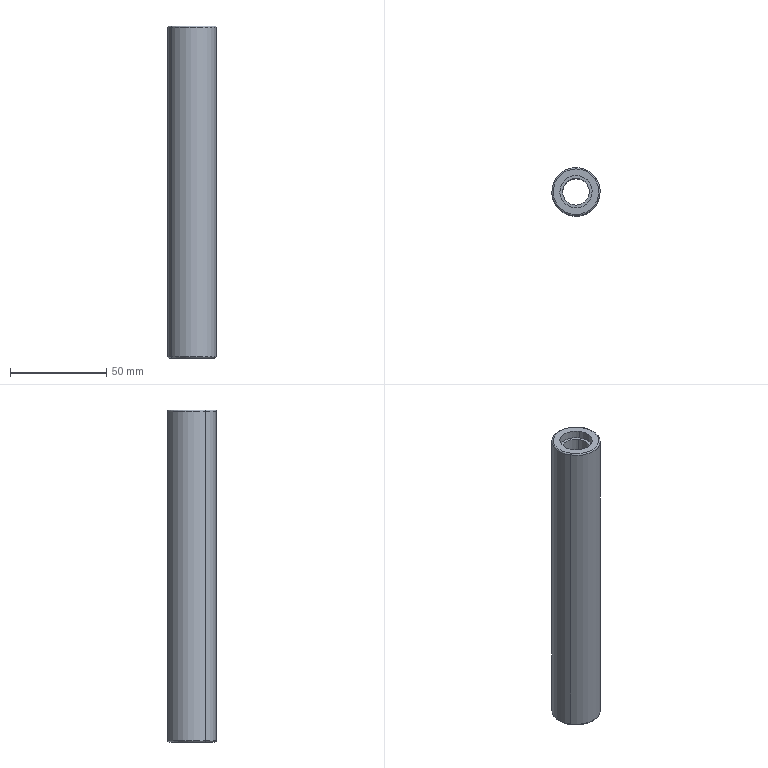Part | SolidWorks | features SplitBody 1 | 1 solid | 16 faces | box 25.2 x 25.2 x 172.9 mm | volume 59034 mm3 | cylinder 8 | torus 4 | plane 4 | commonest cylinder face diameters 16.8 x4 14 x2 25.2 x2
STEP:
#1=CARTESIAN_POINT('',(443.484,236.395,-446.666));
#2=VERTEX_POINT('',#1);
#3=CARTESIAN_POINT('',(463.467,249.323,-446.666));
#4=VERTEX_POINT('',#3);
#5=CARTESIAN_POINT('',(453.475,242.859,-446.666));
#6=DIRECTION('',(0.,0.,-1.));
#7=DIRECTION('',(0.8396,0.5432,0.));
#8=AXIS2_PLACEMENT_3D('',#5,#6,#7);
#9=CIRCLE('',#8,11.9);
#10=EDGE_CURVE('',#2,#4,#9,.T.);
#11=ORIENTED_EDGE('',*,*,#10,.F.);
#12=CARTESIAN_POINT('',(442.896,236.015,-445.966));
#13=VERTEX_POINT('',#12);
#14=CARTESIAN_POINT('',(443.484,236.395,-445.966));
#15=DIRECTION('',(-0.5432,0.8396,0.));
#16=DIRECTION('',(-0.8396,-0.5432,0.));
#17=AXIS2_PLACEMENT_3D('',#14,#15,#16);
#18=CIRCLE('',#17,0.7);
#19=EDGE_CURVE('',#2,#13,#18,.T.);
#20=ORIENTED_EDGE('',*,*,#19,.T.);
#21=CARTESIAN_POINT('',(464.055,249.703,-445.966));
#22=VERTEX_POINT('',#21);
#23=CARTESIAN_POINT('',(453.475,242.859,-445.966));
#24=DIRECTION('',(0.,0.,1.));
#25=DIRECTION('',(0.8396,0.5432,0.));
#26=AXIS2_PLACEMENT_3D('',#23,#24,#25);
#27=CIRCLE('',#26,12.6);
#28=EDGE_CURVE('',#22,#13,#27,.T.);
#29=ORIENTED_EDGE('',*,*,#28,.F.);
#30=CARTESIAN_POINT('',(463.467,249.323,-445.966));
#31=DIRECTION('',(0.5432,-0.8396,0.));
#32=DIRECTION('',(0.8396,0.5432,0.));
#33=AXIS2_PLACEMENT_3D('',#30,#31,#32);
#34=CIRCLE('',#33,0.7);
#35=EDGE_CURVE('',#4,#22,#34,.T.);
#36=ORIENTED_EDGE('',*,*,#35,.F.);
#37=EDGE_LOOP('',(#11,#20,#29,#36));
#38=FACE_OUTER_BOUND('',#37,.T.);
#39=CARTESIAN_POINT('',(453.475,242.859,-445.966));
#40=DIRECTION('',(0.,0.,1.));
#41=DIRECTION('',(0.8396,0.5432,0.));
#42=AXIS2_PLACEMENT_3D('',#39,#40,#41);
#43=TOROIDAL_SURFACE('',#42,11.9,0.7);
#44=ADVANCED_FACE('',(#38),#43,.T.);
#45=CARTESIAN_POINT('',(442.896,236.015,-274.466));
#46=VERTEX_POINT('',#45);
#47=CARTESIAN_POINT('',(464.055,249.703,-274.466));
#48=VERTEX_POINT('',#47);
#49=CARTESIAN_POINT('',(453.475,242.859,-274.466));
#50=DIRECTION('',(0.,0.,-1.));
#51=DIRECTION('',(0.8396,0.5432,0.));
#52=AXIS2_PLACEMENT_3D('',#49,#50,#51);
#53=CIRCLE('',#52,12.6);
#54=EDGE_CURVE('',#46,#48,#53,.T.);
#55=ORIENTED_EDGE('',*,*,#54,.F.);
#56=CARTESIAN_POINT('',(443.484,236.395,-273.766));
#57=VERTEX_POINT('',#56);
#58=CARTESIAN_POINT('',(443.484,236.395,-274.466));
#59=DIRECTION('',(-0.5432,0.8396,0.));
#60=DIRECTION('',(-0.8396,-0.5432,0.));
#61=AXIS2_PLACEMENT_3D('',#58,#59,#60);
#62=CIRCLE('',#61,0.7);
#63=EDGE_CURVE('',#46,#57,#62,.T.);
#64=ORIENTED_EDGE('',*,*,#63,.T.);
#65=CARTESIAN_POINT('',(463.467,249.323,-273.766));
#66=VERTEX_POINT('',#65);
#67=CARTESIAN_POINT('',(453.475,242.859,-273.766));
#68=DIRECTION('',(0.,0.,1.));
#69=DIRECTION('',(0.8396,0.5432,0.));
#70=AXIS2_PLACEMENT_3D('',#67,#68,#69);
#71=CIRCLE('',#70,11.9);
#72=EDGE_CURVE('',#66,#57,#71,.T.);
#73=ORIENTED_EDGE('',*,*,#72,.F.);
#74=CARTESIAN_POINT('',(463.467,249.323,-274.466));
#75=DIRECTION('',(0.5432,-0.8396,0.));
#76=DIRECTION('',(0.8396,0.5432,0.));
#77=AXIS2_PLACEMENT_3D('',#74,#75,#76);
#78=CIRCLE('',#77,0.7);
#79=EDGE_CURVE('',#48,#66,#78,.T.);
#80=ORIENTED_EDGE('',*,*,#79,.F.);
#81=EDGE_LOOP('',(#55,#64,#73,#80));
#82=FACE_OUTER_BOUND('',#81,.T.);
#83=CARTESIAN_POINT('',(453.475,242.859,-274.466));
#84=DIRECTION('',(0.,0.,1.));
#85=DIRECTION('',(0.8396,0.5432,0.));
#86=AXIS2_PLACEMENT_3D('',#83,#84,#85);
#87=TOROIDAL_SURFACE('',#86,11.9,0.7);
#88=ADVANCED_FACE('',(#82),#87,.T.);
#89=CARTESIAN_POINT('',(447.598,239.057,-277.966));
#90=VERTEX_POINT('',#89);
#91=CARTESIAN_POINT('',(459.353,246.661,-277.966));
#92=VERTEX_POINT('',#91);
#93=CARTESIAN_POINT('',(453.475,242.859,-277.966));
#94=DIRECTION('',(0.,0.,1.));
#95=DIRECTION('',(0.8396,0.5432,0.));
#96=AXIS2_PLACEMENT_3D('',#93,#94,#95);
#97=CIRCLE('',#96,7.);
#98=EDGE_CURVE('',#90,#92,#97,.T.);
#99=ORIENTED_EDGE('',*,*,#98,.T.);
#100=CARTESIAN_POINT('',(459.353,246.661,-442.466));
#101=VERTEX_POINT('',#100);
#102=CARTESIAN_POINT('',(459.353,246.661,-273.766));
#103=DIRECTION('',(0.,0.,-1.));
#104=VECTOR('',#103,1000.);
#105=LINE('',#102,#104);
#106=EDGE_CURVE('',#92,#101,#105,.T.);
#107=ORIENTED_EDGE('',*,*,#106,.T.);
#108=CARTESIAN_POINT('',(447.598,239.057,-442.466));
#109=VERTEX_POINT('',#108);
#110=CARTESIAN_POINT('',(453.475,242.859,-442.466));
#111=DIRECTION('',(0.,0.,-1.));
#112=DIRECTION('',(-0.8396,-0.5432,0.));
#113=AXIS2_PLACEMENT_3D('',#110,#111,#112);
#114=CIRCLE('',#113,7.);
#115=EDGE_CURVE('',#101,#109,#114,.T.);
#116=ORIENTED_EDGE('',*,*,#115,.T.);
#117=CARTESIAN_POINT('',(447.598,239.057,-273.766));
#118=DIRECTION('',(0.,0.,-1.));
#119=VECTOR('',#118,1000.);
#120=LINE('',#117,#119);
#121=EDGE_CURVE('',#90,#109,#120,.T.);
#122=ORIENTED_EDGE('',*,*,#121,.F.);
#123=EDGE_LOOP('',(#99,#107,#116,#122));
#124=FACE_OUTER_BOUND('',#123,.T.);
#125=CARTESIAN_POINT('',(453.475,242.859,-273.766));
#126=DIRECTION('',(0.,0.,-1.));
#127=DIRECTION('',(-0.8396,-0.5432,0.));
#128=AXIS2_PLACEMENT_3D('',#125,#126,#127);
#129=CYLINDRICAL_SURFACE('',#128,7.);
#130=ADVANCED_FACE('',(#124),#129,.F.);
#131=CARTESIAN_POINT('',(460.528,247.422,-442.466));
#132=VERTEX_POINT('',#131);
#133=CARTESIAN_POINT('',(446.423,238.296,-442.466));
#134=VERTEX_POINT('',#133);
#135=CARTESIAN_POINT('',(453.475,242.859,-442.466));
#136=DIRECTION('',(0.,0.,-1.));
#137=DIRECTION('',(-0.8396,-0.5432,0.));
#138=AXIS2_PLACEMENT_3D('',#135,#136,#137);
#139=CIRCLE('',#138,8.4);
#140=EDGE_CURVE('',#132,#134,#139,.T.);
#141=ORIENTED_EDGE('',*,*,#140,.F.);
#142=CARTESIAN_POINT('',(460.528,247.422,-446.666));
#143=VERTEX_POINT('',#142);
#144=CARTESIAN_POINT('',(460.528,247.422,-442.466));
#145=DIRECTION('',(0.,0.,-1.));
#146=VECTOR('',#145,1000.);
#147=LINE('',#144,#146);
#148=EDGE_CURVE('',#132,#143,#147,.T.);
#149=ORIENTED_EDGE('',*,*,#148,.T.);
#150=CARTESIAN_POINT('',(446.423,238.296,-446.666));
#151=VERTEX_POINT('',#150);
#152=CARTESIAN_POINT('',(453.475,242.859,-446.666));
#153=DIRECTION('',(0.,0.,-1.));
#154=DIRECTION('',(-0.8396,-0.5432,0.));
#155=AXIS2_PLACEMENT_3D('',#152,#153,#154);
#156=CIRCLE('',#155,8.4);
#157=EDGE_CURVE('',#143,#151,#156,.T.);
#158=ORIENTED_EDGE('',*,*,#157,.T.);
#159=CARTESIAN_POINT('',(446.423,238.296,-442.466));
#160=DIRECTION('',(0.,0.,-1.));
#161=VECTOR('',#160,1000.);
#162=LINE('',#159,#161);
#163=EDGE_CURVE('',#134,#151,#162,.T.);
#164=ORIENTED_EDGE('',*,*,#163,.F.);
#165=EDGE_LOOP('',(#141,#149,#158,#164));
#166=FACE_OUTER_BOUND('',#165,.T.);
#167=CARTESIAN_POINT('',(453.475,242.859,-442.466));
#168=DIRECTION('',(0.,0.,-1.));
#169=DIRECTION('',(-0.8396,-0.5432,0.));
#170=AXIS2_PLACEMENT_3D('',#167,#168,#169);
#171=CYLINDRICAL_SURFACE('',#170,8.4);
#172=ADVANCED_FACE('',(#166),#171,.F.);
#173=CARTESIAN_POINT('',(446.423,238.296,-277.966));
#174=VERTEX_POINT('',#173);
#175=CARTESIAN_POINT('',(460.528,247.422,-277.966));
#176=VERTEX_POINT('',#175);
#177=CARTESIAN_POINT('',(453.475,242.859,-277.966));
#178=DIRECTION('',(0.,0.,1.));
#179=DIRECTION('',(0.8396,0.5432,0.));
#180=AXIS2_PLACEMENT_3D('',#177,#178,#179);
#181=CIRCLE('',#180,8.4);
#182=EDGE_CURVE('',#174,#176,#181,.T.);
#183=ORIENTED_EDGE('',*,*,#182,.F.);
#184=CARTESIAN_POINT('',(446.423,238.296,-273.766));
#185=VERTEX_POINT('',#184);
#186=CARTESIAN_POINT('',(446.423,238.296,-277.966));
#187=DIRECTION('',(0.,0.,1.));
#188=VECTOR('',#187,1000.);
#189=LINE('',#186,#188);
#190=EDGE_CURVE('',#174,#185,#189,.T.);
#191=ORIENTED_EDGE('',*,*,#190,.T.);
#192=CARTESIAN_POINT('',(460.528,247.422,-273.766));
#193=VERTEX_POINT('',#192);
#194=CARTESIAN_POINT('',(453.475,242.859,-273.766));
#195=DIRECTION('',(0.,0.,1.));
#196=DIRECTION('',(0.8396,0.5432,0.));
#197=AXIS2_PLACEMENT_3D('',#194,#195,#196);
#198=CIRCLE('',#197,8.4);
#199=EDGE_CURVE('',#185,#193,#198,.T.);
#200=ORIENTED_EDGE('',*,*,#199,.T.);
#201=CARTESIAN_POINT('',(460.528,247.422,-277.966));
#202=DIRECTION('',(0.,0.,1.));
#203=VECTOR('',#202,1000.);
#204=LINE('',#201,#203);
#205=EDGE_CURVE('',#176,#193,#204,.T.);
#206=ORIENTED_EDGE('',*,*,#205,.F.);
#207=EDGE_LOOP('',(#183,#191,#200,#206));
#208=FACE_OUTER_BOUND('',#207,.T.);
#209=CARTESIAN_POINT('',(453.475,242.859,-277.966));
#210=DIRECTION('',(0.,0.,1.));
#211=DIRECTION('',(0.8396,0.5432,0.));
#212=AXIS2_PLACEMENT_3D('',#209,#210,#211);
#213=CYLINDRICAL_SURFACE('',#212,8.4);
#214=ADVANCED_FACE('',(#208),#213,.F.);
#215=ORIENTED_EDGE('',*,*,#54,.T.);
#216=CARTESIAN_POINT('',(464.055,249.703,-273.766));
#217=DIRECTION('',(0.,0.,-1.));
#218=VECTOR('',#217,1000.);
#219=LINE('',#216,#218);
#220=EDGE_CURVE('',#48,#22,#219,.T.);
#221=ORIENTED_EDGE('',*,*,#220,.T.);
#222=ORIENTED_EDGE('',*,*,#28,.T.);
#223=CARTESIAN_POINT('',(442.896,236.015,-273.766));
#224=DIRECTION('',(0.,0.,-1.));
#225=VECTOR('',#224,1000.);
#226=LINE('',#223,#225);
#227=EDGE_CURVE('',#46,#13,#226,.T.);
#228=ORIENTED_EDGE('',*,*,#227,.F.);
#229=EDGE_LOOP('',(#215,#221,#222,#228));
#230=FACE_OUTER_BOUND('',#229,.T.);
#231=CARTESIAN_POINT('',(453.475,242.859,-273.766));
#232=DIRECTION('',(0.,0.,-1.));
#233=DIRECTION('',(-0.8396,-0.5432,0.));
#234=AXIS2_PLACEMENT_3D('',#231,#232,#233);
#235=CYLINDRICAL_SURFACE('',#234,12.6);
#236=ADVANCED_FACE('',(#230),#235,.T.);
#237=ORIENTED_EDGE('',*,*,#220,.F.);
#238=CARTESIAN_POINT('',(453.475,242.859,-274.466));
#239=DIRECTION('',(0.,0.,-1.));
#240=DIRECTION('',(0.8396,0.5432,0.));
#241=AXIS2_PLACEMENT_3D('',#238,#239,#240);
#242=CIRCLE('',#241,12.6);
#243=EDGE_CURVE('',#48,#46,#242,.T.);
#244=ORIENTED_EDGE('',*,*,#243,.T.);
#245=ORIENTED_EDGE('',*,*,#227,.T.);
#246=CARTESIAN_POINT('',(453.475,242.859,-445.966));
#247=DIRECTION('',(0.,0.,1.));
#248=DIRECTION('',(0.8396,0.5432,0.));
#249=AXIS2_PLACEMENT_3D('',#246,#247,#248);
#250=CIRCLE('',#249,12.6);
#251=EDGE_CURVE('',#13,#22,#250,.T.);
#252=ORIENTED_EDGE('',*,*,#251,.T.);
#253=EDGE_LOOP('',(#237,#244,#245,#252));
#254=FACE_OUTER_BOUND('',#253,.T.);
#255=CARTESIAN_POINT('',(453.475,242.859,-273.766));
#256=DIRECTION('',(0.,0.,-1.));
#257=DIRECTION('',(-0.8396,-0.5432,0.));
#258=AXIS2_PLACEMENT_3D('',#255,#256,#257);
#259=CYLINDRICAL_SURFACE('',#258,12.6);
#260=ADVANCED_FACE('',(#254),#259,.T.);
#261=ORIENTED_EDGE('',*,*,#72,.T.);
#262=CARTESIAN_POINT('',(453.475,242.859,-273.766));
#263=DIRECTION('',(0.,0.,1.));
#264=DIRECTION('',(0.8396,0.5432,0.));
#265=AXIS2_PLACEMENT_3D('',#262,#263,#264);
#266=CIRCLE('',#265,11.9);
#267=EDGE_CURVE('',#57,#66,#266,.T.);
#268=ORIENTED_EDGE('',*,*,#267,.T.);
#269=EDGE_LOOP('',(#261,#268));
#270=FACE_OUTER_BOUND('',#269,.T.);
#271=CARTESIAN_POINT('',(453.475,242.859,-273.766));
#272=DIRECTION('',(0.,0.,1.));
#273=DIRECTION('',(0.8396,0.5432,0.));
#274=AXIS2_PLACEMENT_3D('',#271,#272,#273);
#275=CIRCLE('',#274,8.4);
#276=EDGE_CURVE('',#193,#185,#275,.T.);
#277=ORIENTED_EDGE('',*,*,#276,.F.);
#278=ORIENTED_EDGE('',*,*,#199,.F.);
#279=EDGE_LOOP('',(#277,#278));
#280=FACE_BOUND('',#279,.T.);
#281=CARTESIAN_POINT('',(453.475,242.859,-273.766));
#282=DIRECTION('',(0.,0.,1.));
#283=DIRECTION('',(0.8396,0.5432,0.));
#284=AXIS2_PLACEMENT_3D('',#281,#282,#283);
#285=PLANE('',#284);
#286=ADVANCED_FACE('',(#270,#280),#285,.T.);
#287=CARTESIAN_POINT('',(453.475,242.859,-446.666));
#288=DIRECTION('',(0.,0.,-1.));
#289=DIRECTION('',(0.8396,0.5432,0.));
#290=AXIS2_PLACEMENT_3D('',#287,#288,#289);
#291=CIRCLE('',#290,11.9);
#292=EDGE_CURVE('',#4,#2,#291,.T.);
#293=ORIENTED_EDGE('',*,*,#292,.T.);
#294=ORIENTED_EDGE('',*,*,#10,.T.);
#295=EDGE_LOOP('',(#293,#294));
#296=FACE_OUTER_BOUND('',#295,.T.);
#297=CARTESIAN_POINT('',(453.475,242.859,-446.666));
#298=DIRECTION('',(0.,0.,-1.));
#299=DIRECTION('',(-0.8396,-0.5432,0.));
#300=AXIS2_PLACEMENT_3D('',#297,#298,#299);
#301=CIRCLE('',#300,8.4);
#302=EDGE_CURVE('',#151,#143,#301,.T.);
#303=ORIENTED_EDGE('',*,*,#302,.F.);
#304=ORIENTED_EDGE('',*,*,#157,.F.);
#305=EDGE_LOOP('',(#303,#304));
#306=FACE_BOUND('',#305,.T.);
#307=CARTESIAN_POINT('',(453.475,242.859,-446.666));
#308=DIRECTION('',(0.,0.,1.));
#309=DIRECTION('',(0.8396,0.5432,0.));
#310=AXIS2_PLACEMENT_3D('',#307,#308,#309);
#311=PLANE('',#310);
#312=ADVANCED_FACE('',(#296,#306),#311,.F.);
#313=ORIENTED_EDGE('',*,*,#190,.F.);
#314=CARTESIAN_POINT('',(453.475,242.859,-277.966));
#315=DIRECTION('',(0.,0.,1.));
#316=DIRECTION('',(0.8396,0.5432,0.));
#317=AXIS2_PLACEMENT_3D('',#314,#315,#316);
#318=CIRCLE('',#317,8.4);
#319=EDGE_CURVE('',#176,#174,#318,.T.);
#320=ORIENTED_EDGE('',*,*,#319,.F.);
#321=ORIENTED_EDGE('',*,*,#205,.T.);
#322=ORIENTED_EDGE('',*,*,#276,.T.);
#323=EDGE_LOOP('',(#313,#320,#321,#322));
#324=FACE_OUTER_BOUND('',#323,.T.);
#325=CARTESIAN_POINT('',(453.475,242.859,-277.966));
#326=DIRECTION('',(0.,0.,1.));
#327=DIRECTION('',(0.8396,0.5432,0.));
#328=AXIS2_PLACEMENT_3D('',#325,#326,#327);
#329=CYLINDRICAL_SURFACE('',#328,8.4);
#330=ADVANCED_FACE('',(#324),#329,.F.);
#331=ORIENTED_EDGE('',*,*,#98,.F.);
#332=CARTESIAN_POINT('',(453.475,242.859,-277.966));
#333=DIRECTION('',(0.,0.,1.));
#334=DIRECTION('',(0.8396,0.5432,0.));
#335=AXIS2_PLACEMENT_3D('',#332,#333,#334);
#336=CIRCLE('',#335,7.);
#337=EDGE_CURVE('',#92,#90,#336,.T.);
#338=ORIENTED_EDGE('',*,*,#337,.F.);
#339=EDGE_LOOP('',(#331,#338));
#340=FACE_BOUND('',#339,.T.);
#341=ORIENTED_EDGE('',*,*,#319,.T.);
#342=ORIENTED_EDGE('',*,*,#182,.T.);
#343=EDGE_LOOP('',(#341,#342));
#344=FACE_OUTER_BOUND('',#343,.T.);
#345=CARTESIAN_POINT('',(453.475,242.859,-277.966));
#346=DIRECTION('',(0.,0.,1.));
#347=DIRECTION('',(0.8396,0.5432,0.));
#348=AXIS2_PLACEMENT_3D('',#345,#346,#347);
#349=PLANE('',#348);
#350=ADVANCED_FACE('',(#340,#344),#349,.T.);
#351=ORIENTED_EDGE('',*,*,#148,.F.);
#352=CARTESIAN_POINT('',(453.475,242.859,-442.466));
#353=DIRECTION('',(0.,0.,-1.));
#354=DIRECTION('',(-0.8396,-0.5432,0.));
#355=AXIS2_PLACEMENT_3D('',#352,#353,#354);
#356=CIRCLE('',#355,8.4);
#357=EDGE_CURVE('',#134,#132,#356,.T.);
#358=ORIENTED_EDGE('',*,*,#357,.F.);
#359=ORIENTED_EDGE('',*,*,#163,.T.);
#360=ORIENTED_EDGE('',*,*,#302,.T.);
#361=EDGE_LOOP('',(#351,#358,#359,#360));
#362=FACE_OUTER_BOUND('',#361,.T.);
#363=CARTESIAN_POINT('',(453.475,242.859,-442.466));
#364=DIRECTION('',(0.,0.,-1.));
#365=DIRECTION('',(-0.8396,-0.5432,0.));
#366=AXIS2_PLACEMENT_3D('',#363,#364,#365);
#367=CYLINDRICAL_SURFACE('',#366,8.4);
#368=ADVANCED_FACE('',(#362),#367,.F.);
#369=CARTESIAN_POINT('',(453.475,242.859,-442.466));
#370=DIRECTION('',(0.,0.,-1.));
#371=DIRECTION('',(-0.8396,-0.5432,0.));
#372=AXIS2_PLACEMENT_3D('',#369,#370,#371);
#373=CIRCLE('',#372,7.);
#374=EDGE_CURVE('',#109,#101,#373,.T.);
#375=ORIENTED_EDGE('',*,*,#374,.F.);
#376=ORIENTED_EDGE('',*,*,#115,.F.);
#377=EDGE_LOOP('',(#375,#376));
#378=FACE_BOUND('',#377,.T.);
#379=ORIENTED_EDGE('',*,*,#357,.T.);
#380=ORIENTED_EDGE('',*,*,#140,.T.);
#381=EDGE_LOOP('',(#379,#380));
#382=FACE_OUTER_BOUND('',#381,.T.);
#383=CARTESIAN_POINT('',(453.475,242.859,-442.466));
#384=DIRECTION('',(0.,0.,-1.));
#385=DIRECTION('',(-0.8396,-0.5432,0.));
#386=AXIS2_PLACEMENT_3D('',#383,#384,#385);
#387=PLANE('',#386);
#388=ADVANCED_FACE('',(#378,#382),#387,.T.);
#389=ORIENTED_EDGE('',*,*,#106,.F.);
#390=ORIENTED_EDGE('',*,*,#337,.T.);
#391=ORIENTED_EDGE('',*,*,#121,.T.);
#392=ORIENTED_EDGE('',*,*,#374,.T.);
#393=EDGE_LOOP('',(#389,#390,#391,#392));
#394=FACE_OUTER_BOUND('',#393,.T.);
#395=CARTESIAN_POINT('',(453.475,242.859,-273.766));
#396=DIRECTION('',(0.,0.,-1.));
#397=DIRECTION('',(-0.8396,-0.5432,0.));
#398=AXIS2_PLACEMENT_3D('',#395,#396,#397);
#399=CYLINDRICAL_SURFACE('',#398,7.);
#400=ADVANCED_FACE('',(#394),#399,.F.);
#401=ORIENTED_EDGE('',*,*,#63,.F.);
#402=ORIENTED_EDGE('',*,*,#243,.F.);
#403=ORIENTED_EDGE('',*,*,#79,.T.);
#404=ORIENTED_EDGE('',*,*,#267,.F.);
#405=EDGE_LOOP('',(#401,#402,#403,#404));
#406=FACE_OUTER_BOUND('',#405,.T.);
#407=CARTESIAN_POINT('',(453.475,242.859,-274.466));
#408=DIRECTION('',(0.,0.,1.));
#409=DIRECTION('',(0.8396,0.5432,0.));
#410=AXIS2_PLACEMENT_3D('',#407,#408,#409);
#411=TOROIDAL_SURFACE('',#410,11.9,0.7);
#412=ADVANCED_FACE('',(#406),#411,.T.);
#413=ORIENTED_EDGE('',*,*,#19,.F.);
#414=ORIENTED_EDGE('',*,*,#292,.F.);
#415=ORIENTED_EDGE('',*,*,#35,.T.);
#416=ORIENTED_EDGE('',*,*,#251,.F.);
#417=EDGE_LOOP('',(#413,#414,#415,#416));
#418=FACE_OUTER_BOUND('',#417,.T.);
#419=CARTESIAN_POINT('',(453.475,242.859,-445.966));
#420=DIRECTION('',(0.,0.,1.));
#421=DIRECTION('',(0.8396,0.5432,0.));
#422=AXIS2_PLACEMENT_3D('',#419,#420,#421);
#423=TOROIDAL_SURFACE('',#422,11.9,0.7);
#424=ADVANCED_FACE('',(#418),#423,.T.);
#425=CLOSED_SHELL('',(#44,#88,#130,#172,#214,#236,#260,#286,#312,#330,#350,#368,#388,#400,#412,#424));
#426=MANIFOLD_SOLID_BREP('',#425);
#427=CARTESIAN_POINT('',(0.,0.,0.));
#428=DIRECTION('',(0.,0.,1.));
#429=DIRECTION('',(1.,0.,0.));
#430=AXIS2_PLACEMENT_3D('',#427,#428,#429);
#431=(LENGTH_UNIT()NAMED_UNIT(*)SI_UNIT(.MILLI.,.METRE.));
#432=UNCERTAINTY_MEASURE_WITH_UNIT(LENGTH_MEASURE(0.00001),#431,'','');
#433=(NAMED_UNIT(*)PLANE_ANGLE_UNIT()SI_UNIT($,.RADIAN.));
#434=(NAMED_UNIT(*)SI_UNIT($,.STERADIAN.)SOLID_ANGLE_UNIT());
#435=(GEOMETRIC_REPRESENTATION_CONTEXT(3)GLOBAL_UNCERTAINTY_ASSIGNED_CONTEXT((#432))GLOBAL_UNIT_ASSIGNED_CONTEXT((#431,#433,#434))REPRESENTATION_CONTEXT('',''));
#436=ADVANCED_BREP_SHAPE_REPRESENTATION('',(#426,#430),#435);